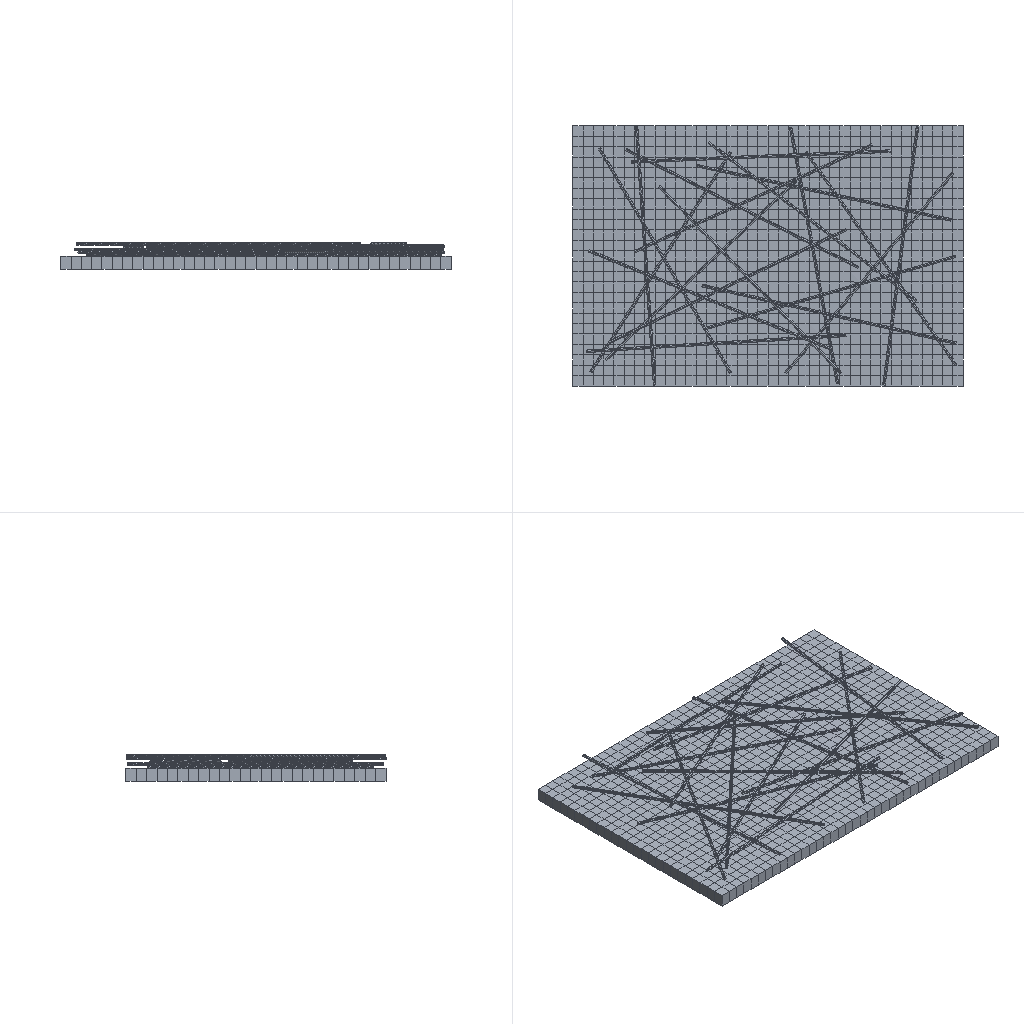Simulation study | abaqus
Set-up summary:
category,name,step,type,value,unit,region
solver,abaqus
solver,version,,,Abaqus/Explicit 2020
units,not stated in the deck,,not stated
analysis,deck,,transient,transient
load_step,Step-1,Step-1,transient
load_step,Step-2,Step-2,transient
load_step,requested,,,2
mesh,nodes,,,6474
mesh,elements,,,2850
element_type,C3D8R,,solid,2850
load,load commands in deck,,count,3
bc,support commands in deck,,count,18
material,JITI,,in results
material,MATERIAL-1,,in results
check,setup vs results,,match,"per instance, exact: element labels, types and connectivity; labels of the nodes the elements use; coordinates of those nodes at SINGLE_PRECISION in 16 of 20 instance(s)"
Abaqus input file, long lists of numbers shortened:
*Heading
** Job name: Job-2 Model name: Model-1-Copy
** Generated by: Abaqus/CAE 2020
*Preprint, echo=NO, model=NO, history=NO, contact=NO
**
** PARTS
**
*Part, name=P1111-1
*End Part
**
*Part, name=P1111-2
*End Part
**
*Part, name=P1111-3
*End Part
**
*Part, name=P1111-4
*End Part
**
*Part, name=P1111-5
*End Part
**
*Part, name=P1111-6
*End Part
**
*Part, name=P1111-7
*End Part
**
*Part, name=P1111-8
*End Part
**
*Part, name=P1111-9
*End Part
**
*Part, name=P1111-10
*End Part
**
*Part, name=P1111-11
*End Part
**
*Part, name=P1111-12
*End Part
**
*Part, name=P1111-13
*End Part
**
*Part, name=P1111-14
*End Part
**
*Part, name=P1111-15
*End Part
**
*Part, name=P1111-16
*End Part
**
*Part, name=P1111-17
*End Part
**
*Part, name=P1111-18
*End Part
**
*Part, name=P1111-19
*End Part
**
*Part, name=P1111-20
*End Part
**
**
** ASSEMBLY
**
*Assembly, name=Assembly
**
*Instance, name=P1111-1-1, part=P1111-1
*Node
      1,  -42.19,   54.229,           0.
      2,  -42.19,   50.229,           0.
** (2026 more lines like these left out)
*Element, type=C3D8R
  1,   53,   54,   80,   79,    1,    2,   28,   27
  2,   54,   55,   81,   80,    2,    3,   29,   28
** (948 more lines like these left out)
*Nset, nset=Set-1, generate
    1,  2028,     1
*Elset, elset=Set-1, generate
   1,  950,    1
** Section: jiti
*Solid Section, elset=Set-1, material=jiti
,
*End Instance
**
*Instance, name=P1111-2-1, part=P1111-2
*Node
      1,  -31.669,   45.76,   5.139
      2,  -31.974,   45.582,   4.992
** (232 more lines like these left out)
*Element, type=C3D8R
  1,   1,   9,   3,   2,  10,  18,  12,  11
  2,   7,   6,   5,   9,  16,  15,  14,  18
** (98 more lines like these left out)
*Nset, nset=Set-1, generate
   1,  234,    1
*Elset, elset=Set-1, generate
   1,  100,    1
** Section: yuanzhu
*Solid Section, elset=Set-1, material=Material-1
,
*End Instance
**
*Instance, name=P1111-3-1, part=P1111-3
*Node
      1,   104.08,   35.777,   5.139
      2,    103.809,   36.004,   4.992
** (232 more lines like these left out)
*Element, type=C3D8R
  1,   2,   1,   8,   9,  11,  10,  17,  18
  2,   2,   9,   4,   3,  11,  18,  13,  12
** (98 more lines like these left out)
*Nset, nset=Set-1, generate
   1,  234,    1
*Elset, elset=Set-1, generate
   1,  100,    1
** Section: yuanzhu
*Solid Section, elset=Set-1, material=Material-1
,
*End Instance
**
*Instance, name=P1111-4-1, part=P1111-4
*Node
      1,  -21.552,   45.409,   5.139
      2,  -21.712,   45.094,   4.992
** (232 more lines like these left out)
*Element, type=C3D8R
  1,   6,   9,   8,   7,  15,  18,  17,  16
  2,   4,   3,   2,   9,  13,  12,  11,  18
** (98 more lines like these left out)
*Nset, nset=Set-1, generate
   1,  234,    1
*Elset, elset=Set-1, generate
   1,  100,    1
** Section: yuanzhu
*Solid Section, elset=Set-1, material=Material-1
,
*End Instance
**
*Instance, name=P1111-5-1, part=P1111-5
*Node
      1,   -35.497,  -40.087,   6.265
      2,  -35.199,  -40.277,   6.118
** (232 more lines like these left out)
*Element, type=C3D8R
  1,   4,   9,   6,   5,  13,  18,  15,  14
  2,   8,   7,   6,   9,  17,  16,  15,  18
** (98 more lines like these left out)
*Nset, nset=Set-1, generate
   1,  234,    1
*Elset, elset=Set-1, generate
   1,  100,    1
** Section: yuanzhu
*Solid Section, elset=Set-1, material=Material-1
,
*End Instance
**
*Instance, name=P1111-6-1, part=P1111-6
*Node
      1,   104.726,  -37.897,   6.265
      2,   105.015,  -37.693,   6.118
** (232 more lines like these left out)
*Element, type=C3D8R
  1,   6,   9,   8,   7,  15,  18,  17,  16
  2,   6,   5,   4,   9,  15,  14,  13,  18
** (98 more lines like these left out)
*Nset, nset=Set-1, generate
   1,  234,    1
*Elset, elset=Set-1, generate
   1,  100,    1
** Section: yuanzhu
*Solid Section, elset=Set-1, material=Material-1
,
*End Instance
**
*Instance, name=P1111-7-1, part=P1111-7
*Node
      1,   59.185,  -44.893,   6.265
      2,   59.533,  -44.83,   6.118
** (232 more lines like these left out)
*Element, type=C3D8R
  1,   4,   3,   2,   9,  13,  12,  11,  18
  2,   4,   9,   6,   5,  13,  18,  15,  14
** (98 more lines like these left out)
*Nset, nset=Set-1, generate
   1,  234,    1
*Elset, elset=Set-1, generate
   1,  100,    1
** Section: yuanzhu
*Solid Section, elset=Set-1, material=Material-1
,
*End Instance
**
*Instance, name=P1111-8-1, part=P1111-8
*Node
      1,  -29.698,  -35.221,   6.303
      2,   -29.456,  -35.479,    6.156
** (232 more lines like these left out)
*Element, type=C3D8R
  1,   8,   7,   6,   9,  17,  16,  15,  18
  2,   8,   9,   2,   1,  17,  18,  11,  10
** (98 more lines like these left out)
*Nset, nset=Set-1, generate
   1,  234,    1
*Elset, elset=Set-1, generate
   1,  100,    1
** Section: yuanzhu
*Solid Section, elset=Set-1, material=Material-1
,
*End Instance
**
*Instance, name=P1111-9-1, part=P1111-9
*Node
      1,  -37.063,  -32.075,   7.313
      2,  -37.041,  -32.428,   7.166
** (232 more lines like these left out)
*Element, type=C3D8R
  1,   6,   9,   8,   7,  15,  18,  17,  16
  2,   4,   3,   2,   9,  13,  12,  11,  18
** (98 more lines like these left out)
*Nset, nset=Set-1, generate
   1,  234,    1
*Elset, elset=Set-1, generate
   1,  100,    1
** Section: yuanzhu
*Solid Section, elset=Set-1, material=Material-1
,
*End Instance
**
*Instance, name=P1111-10-1, part=P1111-10
*Node
      1,  -27.663,  -28.386,   7.313
      2,  -27.511,  -28.705,   7.166
** (232 more lines like these left out)
*Element, type=C3D8R
  1,   2,   1,   8,   9,  11,  10,  17,  18
  2,   4,   9,   6,   5,  13,  18,  15,  14
** (98 more lines like these left out)
*Nset, nset=Set-1, generate
   1,  234,    1
*Elset, elset=Set-1, generate
   1,  100,    1
** Section: yuanzhu
*Solid Section, elset=Set-1, material=Material-1
,
*End Instance
**
*Instance, name=P1111-11-1, part=P1111-11
*Node
      1,   5.398,   39.306,   7.313
      2,   5.324,   38.96,   7.166
** (232 more lines like these left out)
*Element, type=C3D8R
  1,   6,   9,   8,   7,  15,  18,  17,  16
  2,   8,   9,   2,   1,  17,  18,  11,  10
** (98 more lines like these left out)
*Nset, nset=Set-1, generate
   1,  234,    1
*Elset, elset=Set-1, generate
   1,  100,    1
** Section: yuanzhu
*Solid Section, elset=Set-1, material=Material-1
,
*End Instance
**
*Instance, name=P1111-12-1, part=P1111-12
*Node
      1,   7.535,  -6.803,   8.533
      2,   7.456,  -7.148,    8.386
** (232 more lines like these left out)
*Element, type=C3D8R
  1,   5,   9,   7,   6,  14,  18,  16,  15
  2,   1,   8,   7,   9,  10,  17,  16,  18
** (98 more lines like these left out)
*Nset, nset=Set-1, generate
   1,  234,    1
*Elset, elset=Set-1, generate
   1,  100,    1
** Section: yuanzhu
*Solid Section, elset=Set-1, material=Material-1
,
*End Instance
**
*Instance, name=P1111-13-1, part=P1111-13
*Node
      1,  -8.713,   31.118,   8.404
      2,  -8.966,    30.871,   8.258
** (232 more lines like these left out)
*Element, type=C3D8R
  1,   4,   9,   6,   5,  13,  18,  15,  14
  2,   8,   9,   2,   1,  17,  18,  11,  10
** (98 more lines like these left out)
*Nset, nset=Set-1, generate
   1,  234,    1
*Elset, elset=Set-1, generate
   1,  100,    1
** Section: yuanzhu
*Solid Section, elset=Set-1, material=Material-1
,
*End Instance
**
*Instance, name=P1111-14-1, part=P1111-14
*Node
      1,   90.585,   53.756,   9.437
      2,   90.235,   53.802,   9.29
** (232 more lines like these left out)
*Element, type=C3D8R
  1,   5,   9,   7,   6,  14,  18,  16,  15
  2,   1,   9,   3,   2,  10,  18,  12,  11
** (98 more lines like these left out)
*Nset, nset=Set-1, generate
   1,  234,    1
*Elset, elset=Set-1, generate
   1,  100,    1
** Section: yuanzhu
*Solid Section, elset=Set-1, material=Material-1
,
*End Instance
**
*Instance, name=P1111-15-1, part=P1111-15
*Node
      1,  -17.369,   53.979,   8.404
      2,  -17.722,    53.955,   8.258
** (232 more lines like these left out)
*Element, type=C3D8R
  1,   7,   6,   5,   9,  16,  15,  14,  18
  2,   5,   4,   3,   9,  14,  13,  12,  18
** (98 more lines like these left out)
*Nset, nset=Set-1, generate
   1,  234,    1
*Elset, elset=Set-1, generate
   1,  100,    1
** Section: yuanzhu
*Solid Section, elset=Set-1, material=Material-1
,
*End Instance
**
*Instance, name=P1111-16-1, part=P1111-16
*Node
      1,   10.313,   47.989,   8.404
      2,   10.099,   47.707,   8.258
** (232 more lines like these left out)
*Element, type=C3D8R
  1,   1,   9,   3,   2,  10,  18,  12,  11
  2,   7,   6,   5,   9,  16,  15,  14,  18
** (98 more lines like these left out)
*Nset, nset=Set-1, generate
   1,  234,    1
*Elset, elset=Set-1, generate
   1,  100,    1
** Section: yuanzhu
*Solid Section, elset=Set-1, material=Material-1
,
*End Instance
**
*Instance, name=P1111-17-1, part=P1111-17
*Node
      1,  -35.913,   6.512,   9.437
      2,   -36.045,   6.185,   9.29
** (232 more lines like these left out)
*Element, type=C3D8R
  1,   5,   9,   7,   6,  14,  18,  16,  15
  2,   5,   4,   3,   9,  14,  13,  12,  18
** (98 more lines like these left out)
*Nset, nset=Set-1, generate
   1,  234,    1
*Elset, elset=Set-1, generate
   1,  100,    1
** Section: yuanzhu
*Solid Section, elset=Set-1, material=Material-1
,
*End Instance
**
*Instance, name=P1111-18-1, part=P1111-18
*Node
      1,  -18.626,   6.193,   9.437
      2,  -18.481,   5.871,   9.29
** (232 more lines like these left out)
*Element, type=C3D8R
  1,   7,   6,   5,   9,  16,  15,  14,  18
  2,   1,   8,   7,   9,  10,  17,  16,  18
** (98 more lines like these left out)
*Nset, nset=Set-1, generate
   1,  234,    1
*Elset, elset=Set-1, generate
   1,  100,    1
** Section: yuanzhu
*Solid Section, elset=Set-1, material=Material-1
,
*End Instance
**
*Instance, name=P1111-19-1, part=P1111-19
*Node
      1,  -19.828,   40.731,   7.313
      2,  -19.814,   40.378,   7.166
** (232 more lines like these left out)
*Element, type=C3D8R
  1,   1,   9,   3,   2,  10,  18,  12,  11
  2,   7,   6,   5,   9,  16,  15,  14,  18
** (98 more lines like these left out)
*Nset, nset=Set-1, generate
   1,  234,    1
*Elset, elset=Set-1, generate
   1,  100,    1
** Section: yuanzhu
*Solid Section, elset=Set-1, material=Material-1
,
*End Instance
**
*Instance, name=P1111-20-1, part=P1111-20
*Node
      1,   8.641,  -23.322,   7.313
      2,   8.739,   -23.661,   7.166
** (232 more lines like these left out)
*Element, type=C3D8R
  1,   2,   1,   8,   9,  11,  10,  17,  18
  2,   4,   9,   6,   5,  13,  18,  15,  14
** (98 more lines like these left out)
*Nset, nset=Set-1, generate
   1,  234,    1
*Elset, elset=Set-1, generate
   1,  100,    1
** Section: yuanzhu
*Solid Section, elset=Set-1, material=Material-1
,
*End Instance
**
*Nset, nset=Set-1, instance=P1111-2-1, generate
   1,  234,    1
*Nset, nset=Set-1, instance=P1111-3-1, generate
   1,  234,    1
*Nset, nset=Set-1, instance=P1111-4-1, generate
   1,  234,    1
*Nset, nset=Set-1, instance=P1111-8-1, generate
   1,  234,    1
*Nset, nset=Set-1, instance=P1111-16-1, generate
   1,  234,    1
*Nset, nset=Set-1, instance=P1111-12-1, generate
   1,  234,    1
*Nset, nset=Set-1, instance=P1111-20-1, generate
   1,  234,    1
*Nset, nset=Set-1, instance=P1111-6-1, generate
   1,  234,    1
*Nset, nset=Set-1, instance=P1111-10-1, generate
   1,  234,    1
*Nset, nset=Set-1, instance=P1111-18-1, generate
   1,  234,    1
*Nset, nset=Set-1, instance=P1111-14-1, generate
   1,  234,    1
*Nset, nset=Set-1, instance=P1111-5-1, generate
   1,  234,    1
*Nset, nset=Set-1, instance=P1111-9-1, generate
   1,  234,    1
*Nset, nset=Set-1, instance=P1111-17-1, generate
   1,  234,    1
*Nset, nset=Set-1, instance=P1111-13-1, generate
   1,  234,    1
*Nset, nset=Set-1, instance=P1111-7-1, generate
   1,  234,    1
*Nset, nset=Set-1, instance=P1111-11-1, generate
   1,  234,    1
*Nset, nset=Set-1, instance=P1111-19-1, generate
   1,  234,    1
*Nset, nset=Set-1, instance=P1111-15-1, generate
   1,  234,    1
*Elset, elset=Set-1, instance=P1111-2-1, generate
   1,  100,    1
*Elset, elset=Set-1, instance=P1111-3-1, generate
   1,  100,    1
*Elset, elset=Set-1, instance=P1111-4-1, generate
   1,  100,    1
*Elset, elset=Set-1, instance=P1111-8-1, generate
   1,  100,    1
*Elset, elset=Set-1, instance=P1111-16-1, generate
   1,  100,    1
*Elset, elset=Set-1, instance=P1111-12-1, generate
   1,  100,    1
*Elset, elset=Set-1, instance=P1111-20-1, generate
   1,  100,    1
*Elset, elset=Set-1, instance=P1111-6-1, generate
   1,  100,    1
*Elset, elset=Set-1, instance=P1111-10-1, generate
   1,  100,    1
*Elset, elset=Set-1, instance=P1111-18-1, generate
   1,  100,    1
*Elset, elset=Set-1, instance=P1111-14-1, generate
   1,  100,    1
*Elset, elset=Set-1, instance=P1111-5-1, generate
   1,  100,    1
*Elset, elset=Set-1, instance=P1111-9-1, generate
   1,  100,    1
*Elset, elset=Set-1, instance=P1111-17-1, generate
   1,  100,    1
*Elset, elset=Set-1, instance=P1111-13-1, generate
   1,  100,    1
*Elset, elset=Set-1, instance=P1111-7-1, generate
   1,  100,    1
*Elset, elset=Set-1, instance=P1111-11-1, generate
   1,  100,    1
*Elset, elset=Set-1, instance=P1111-19-1, generate
   1,  100,    1
*Elset, elset=Set-1, instance=P1111-15-1, generate
   1,  100,    1
*Nset, nset=Set-2, instance=P1111-1-1, generate
  1,  52,   1
*Elset, elset=Set-2, instance=P1111-1-1, generate
  1,  25,   1
*Nset, nset=Set-3, instance=P1111-1-1, generate
 1977,  2028,     1
*Elset, elset=Set-3, instance=P1111-1-1, generate
 926,  950,    1
*Nset, nset=Set-4, instance=P1111-1-1
    1,    2,    3,    4,    5,    6,    7,    8,    9,   10,   11,   12,   13,   14,   15,   16
   17,   18,   19,   20,   21,   22,   23,   24,   25,   26,   53,   54,   55,   56,   57,   58
** (62 more lines like these left out)
*Elset, elset=Set-4, instance=P1111-1-1, generate
   1,  950,    1
*Elset, elset=_m_Surf-1_S5, internal, instance=P1111-2-1, generate
  1,  97,   4
*Elset, elset=_m_Surf-1_S5, internal, instance=P1111-3-1
  2,  3,  6,  7, 10, 11, 14, 15, 18, 19, 22, 23, 26, 27, 30, 31
 34, 35, 38, 39, 42, 43, 46, 47, 50, 51, 54, 55, 58, 59, 62, 63
** (2 more lines like these left out)
*Elset, elset=_m_Surf-1_S5, internal, instance=P1111-4-1
   1,   3,   4,   5,   7,   8,   9,  11,  12,  13,  15,  16,  17,  19,  20,  21
  23,  24,  25,  27,  28,  29,  31,  32,  33,  35,  36,  37,  39,  40,  41,  43
** (3 more lines like these left out)
*Elset, elset=_m_Surf-1_S5, internal, instance=P1111-8-1
   2,   3,   4,   6,   7,   8,  10,  11,  12,  14,  15,  16,  18,  19,  20,  22
  23,  24,  26,  27,  28,  30,  31,  32,  34,  35,  36,  38,  39,  40,  42,  43
** (3 more lines like these left out)
*Elset, elset=_m_Surf-1_S5, internal, instance=P1111-16-1, generate
  1,  99,   2
*Elset, elset=_m_Surf-1_S5, internal, instance=P1111-12-1
   1,   4,   5,   8,   9,  12,  13,  16,  17,  20,  21,  24,  25,  28,  29,  32
  33,  36,  37,  40,  41,  44,  45,  48,  49,  52,  53,  56,  57,  60,  61,  64
** (2 more lines like these left out)
*Elset, elset=_m_Surf-1_S5, internal, instance=P1111-20-1
  2,  3,  6,  7, 10, 11, 14, 15, 18, 19, 22, 23, 26, 27, 30, 31
 34, 35, 38, 39, 42, 43, 46, 47, 50, 51, 54, 55, 58, 59, 62, 63
** (2 more lines like these left out)
*Elset, elset=_m_Surf-1_S5, internal, instance=P1111-6-1
   1,   3,   4,   5,   7,   8,   9,  11,  12,  13,  15,  16,  17,  19,  20,  21
  23,  24,  25,  27,  28,  29,  31,  32,  33,  35,  36,  37,  39,  40,  41,  43
** (3 more lines like these left out)
*Elset, elset=_m_Surf-1_S5, internal, instance=P1111-10-1
  2,  3,  6,  7, 10, 11, 14, 15, 18, 19, 22, 23, 26, 27, 30, 31
 34, 35, 38, 39, 42, 43, 46, 47, 50, 51, 54, 55, 58, 59, 62, 63
** (2 more lines like these left out)
*Elset, elset=_m_Surf-1_S5, internal, instance=P1111-18-1, generate
  3,  99,   4
*Elset, elset=_m_Surf-1_S5, internal, instance=P1111-14-1
  1,  2,  3,  5,  6,  7,  9, 10, 11, 13, 14, 15, 17, 18, 19, 21
 22, 23, 25, 26, 27, 29, 30, 31, 33, 34, 35, 37, 38, 39, 41, 42
** (3 more lines like these left out)
*Elset, elset=_m_Surf-1_S5, internal, instance=P1111-5-1, generate
  1,  97,   4
*Elset, elset=_m_Surf-1_S5, internal, instance=P1111-9-1
   1,   3,   4,   5,   7,   8,   9,  11,  12,  13,  15,  16,  17,  19,  20,  21
  23,  24,  25,  27,  28,  29,  31,  32,  33,  35,  36,  37,  39,  40,  41,  43
** (3 more lines like these left out)
*Elset, elset=_m_Surf-1_S5, internal, instance=P1111-17-1
   1,   4,   5,   8,   9,  12,  13,  16,  17,  20,  21,  24,  25,  28,  29,  32
  33,  36,  37,  40,  41,  44,  45,  48,  49,  52,  53,  56,  57,  60,  61,  64
** (2 more lines like these left out)
*Elset, elset=_m_Surf-1_S5, internal, instance=P1111-13-1
  1,  2,  3,  5,  6,  7,  9, 10, 11, 13, 14, 15, 17, 18, 19, 21
 22, 23, 25, 26, 27, 29, 30, 31, 33, 34, 35, 37, 38, 39, 41, 42
** (3 more lines like these left out)
*Elset, elset=_m_Surf-1_S5, internal, instance=P1111-7-1, generate
  2,  98,   4
*Elset, elset=_m_Surf-1_S5, internal, instance=P1111-11-1, generate
   1,  100,    1
*Elset, elset=_m_Surf-1_S5, internal, instance=P1111-19-1, generate
  1,  99,   2
*Elset, elset=_m_Surf-1_S5, internal, instance=P1111-15-1, generate
   4,  100,    4
*Elset, elset=_m_Surf-1_S6, internal, instance=P1111-2-1, generate
  1,  97,   4
*Elset, elset=_m_Surf-1_S6, internal, instance=P1111-3-1
  2,  3,  6,  7, 10, 11, 14, 15, 18, 19, 22, 23, 26, 27, 30, 31
 34, 35, 38, 39, 42, 43, 46, 47, 50, 51, 54, 55, 58, 59, 62, 63
** (2 more lines like these left out)
*Elset, elset=_m_Surf-1_S6, internal, instance=P1111-4-1
   1,   3,   4,   5,   7,   8,   9,  11,  12,  13,  15,  16,  17,  19,  20,  21
  23,  24,  25,  27,  28,  29,  31,  32,  33,  35,  36,  37,  39,  40,  41,  43
** (3 more lines like these left out)
*Elset, elset=_m_Surf-1_S6, internal, instance=P1111-8-1
   2,   3,   4,   6,   7,   8,  10,  11,  12,  14,  15,  16,  18,  19,  20,  22
  23,  24,  26,  27,  28,  30,  31,  32,  34,  35,  36,  38,  39,  40,  42,  43
** (3 more lines like these left out)
*Elset, elset=_m_Surf-1_S6, internal, instance=P1111-16-1, generate
  1,  99,   2
*Elset, elset=_m_Surf-1_S6, internal, instance=P1111-12-1
   1,   4,   5,   8,   9,  12,  13,  16,  17,  20,  21,  24,  25,  28,  29,  32
  33,  36,  37,  40,  41,  44,  45,  48,  49,  52,  53,  56,  57,  60,  61,  64
** (2 more lines like these left out)
*Elset, elset=_m_Surf-1_S6, internal, instance=P1111-20-1
  2,  3,  6,  7, 10, 11, 14, 15, 18, 19, 22, 23, 26, 27, 30, 31
 34, 35, 38, 39, 42, 43, 46, 47, 50, 51, 54, 55, 58, 59, 62, 63
** (2 more lines like these left out)
*Elset, elset=_m_Surf-1_S6, internal, instance=P1111-6-1
   1,   3,   4,   5,   7,   8,   9,  11,  12,  13,  15,  16,  17,  19,  20,  21
  23,  24,  25,  27,  28,  29,  31,  32,  33,  35,  36,  37,  39,  40,  41,  43
** (3 more lines like these left out)
*Elset, elset=_m_Surf-1_S6, internal, instance=P1111-10-1
  2,  3,  6,  7, 10, 11, 14, 15, 18, 19, 22, 23, 26, 27, 30, 31
 34, 35, 38, 39, 42, 43, 46, 47, 50, 51, 54, 55, 58, 59, 62, 63
** (2 more lines like these left out)
*Elset, elset=_m_Surf-1_S6, internal, instance=P1111-18-1, generate
  3,  99,   4
*Elset, elset=_m_Surf-1_S6, internal, instance=P1111-14-1
  1,  2,  3,  5,  6,  7,  9, 10, 11, 13, 14, 15, 17, 18, 19, 21
 22, 23, 25, 26, 27, 29, 30, 31, 33, 34, 35, 37, 38, 39, 41, 42
** (3 more lines like these left out)
*Elset, elset=_m_Surf-1_S6, internal, instance=P1111-5-1, generate
  1,  97,   4
*Elset, elset=_m_Surf-1_S6, internal, instance=P1111-9-1
   1,   3,   4,   5,   7,   8,   9,  11,  12,  13,  15,  16,  17,  19,  20,  21
  23,  24,  25,  27,  28,  29,  31,  32,  33,  35,  36,  37,  39,  40,  41,  43
** (3 more lines like these left out)
*Elset, elset=_m_Surf-1_S6, internal, instance=P1111-17-1
   1,   4,   5,   8,   9,  12,  13,  16,  17,  20,  21,  24,  25,  28,  29,  32
  33,  36,  37,  40,  41,  44,  45,  48,  49,  52,  53,  56,  57,  60,  61,  64
** (2 more lines like these left out)
*Elset, elset=_m_Surf-1_S6, internal, instance=P1111-13-1
  1,  2,  3,  5,  6,  7,  9, 10, 11, 13, 14, 15, 17, 18, 19, 21
 22, 23, 25, 26, 27, 29, 30, 31, 33, 34, 35, 37, 38, 39, 41, 42
** (3 more lines like these left out)
*Elset, elset=_m_Surf-1_S6, internal, instance=P1111-7-1, generate
  2,  98,   4
*Elset, elset=_m_Surf-1_S6, internal, instance=P1111-11-1, generate
   1,  100,    1
*Elset, elset=_m_Surf-1_S6, internal, instance=P1111-19-1, generate
  1,  99,   2
*Elset, elset=_m_Surf-1_S6, internal, instance=P1111-15-1, generate
   4,  100,    4
*Elset, elset=_m_Surf-1_S3, internal, instance=P1111-2-1
   2,   3,   4,   6,   7,   8,  10,  11,  12,  14,  15,  16,  18,  19,  20,  22
  23,  24,  26,  27,  28,  30,  31,  32,  34,  35,  36,  38,  39,  40,  42,  43
** (3 more lines like these left out)
*Elset, elset=_m_Surf-1_S3, internal, instance=P1111-3-1
   1,   4,   5,   8,   9,  12,  13,  16,  17,  20,  21,  24,  25,  28,  29,  32
  33,  36,  37,  40,  41,  44,  45,  48,  49,  52,  53,  56,  57,  60,  61,  64
** (2 more lines like these left out)
*Elset, elset=_m_Surf-1_S3, internal, instance=P1111-4-1, generate
  2,  98,   4
*Elset, elset=_m_Surf-1_S3, internal, instance=P1111-8-1, generate
  1,  97,   4
*Elset, elset=_m_Surf-1_S3, internal, instance=P1111-16-1, generate
   2,  100,    2
*Elset, elset=_m_Surf-1_S3, internal, instance=P1111-12-1
  2,  3,  6,  7, 10, 11, 14, 15, 18, 19, 22, 23, 26, 27, 30, 31
 34, 35, 38, 39, 42, 43, 46, 47, 50, 51, 54, 55, 58, 59, 62, 63
** (2 more lines like these left out)
*Elset, elset=_m_Surf-1_S3, internal, instance=P1111-20-1
   1,   4,   5,   8,   9,  12,  13,  16,  17,  20,  21,  24,  25,  28,  29,  32
  33,  36,  37,  40,  41,  44,  45,  48,  49,  52,  53,  56,  57,  60,  61,  64
** (2 more lines like these left out)
*Elset, elset=_m_Surf-1_S3, internal, instance=P1111-6-1, generate
  2,  98,   4
*Elset, elset=_m_Surf-1_S3, internal, instance=P1111-10-1
   1,   4,   5,   8,   9,  12,  13,  16,  17,  20,  21,  24,  25,  28,  29,  32
  33,  36,  37,  40,  41,  44,  45,  48,  49,  52,  53,  56,  57,  60,  61,  64
** (2 more lines like these left out)
*Elset, elset=_m_Surf-1_S3, internal, instance=P1111-18-1
   1,   2,   4,   5,   6,   8,   9,  10,  12,  13,  14,  16,  17,  18,  20,  21
  22,  24,  25,  26,  28,  29,  30,  32,  33,  34,  36,  37,  38,  40,  41,  42
** (3 more lines like these left out)
*Elset, elset=_m_Surf-1_S3, internal, instance=P1111-14-1, generate
   4,  100,    4
*Elset, elset=_m_Surf-1_S3, internal, instance=P1111-5-1
   2,   3,   4,   6,   7,   8,  10,  11,  12,  14,  15,  16,  18,  19,  20,  22
  23,  24,  26,  27,  28,  30,  31,  32,  34,  35,  36,  38,  39,  40,  42,  43
** (3 more lines like these left out)
*Elset, elset=_m_Surf-1_S3, internal, instance=P1111-9-1, generate
  2,  98,   4
*Elset, elset=_m_Surf-1_S3, internal, instance=P1111-17-1
  2,  3,  6,  7, 10, 11, 14, 15, 18, 19, 22, 23, 26, 27, 30, 31
 34, 35, 38, 39, 42, 43, 46, 47, 50, 51, 54, 55, 58, 59, 62, 63
** (2 more lines like these left out)
*Elset, elset=_m_Surf-1_S3, internal, instance=P1111-13-1, generate
   4,  100,    4
*Elset, elset=_m_Surf-1_S3, internal, instance=P1111-7-1
   1,   3,   4,   5,   7,   8,   9,  11,  12,  13,  15,  16,  17,  19,  20,  21
  23,  24,  25,  27,  28,  29,  31,  32,  33,  35,  36,  37,  39,  40,  41,  43
** (3 more lines like these left out)
*Elset, elset=_m_Surf-1_S3, internal, instance=P1111-19-1, generate
   2,  100,    2
*Elset, elset=_m_Surf-1_S3, internal, instance=P1111-15-1
  1,  2,  3,  5,  6,  7,  9, 10, 11, 13, 14, 15, 17, 18, 19, 21
 22, 23, 25, 26, 27, 29, 30, 31, 33, 34, 35, 37, 38, 39, 41, 42
** (3 more lines like these left out)
*Elset, elset=_m_Surf-1_S4, internal, instance=P1111-2-1
   2,   3,   4,   6,   7,   8,  10,  11,  12,  14,  15,  16,  18,  19,  20,  22
  23,  24,  26,  27,  28,  30,  31,  32,  34,  35,  36,  38,  39,  40,  42,  43
** (3 more lines like these left out)
*Elset, elset=_m_Surf-1_S4, internal, instance=P1111-3-1
   1,   4,   5,   8,   9,  12,  13,  16,  17,  20,  21,  24,  25,  28,  29,  32
  33,  36,  37,  40,  41,  44,  45,  48,  49,  52,  53,  56,  57,  60,  61,  64
** (2 more lines like these left out)
*Elset, elset=_m_Surf-1_S4, internal, instance=P1111-4-1, generate
  2,  98,   4
*Elset, elset=_m_Surf-1_S4, internal, instance=P1111-8-1, generate
  1,  97,   4
*Elset, elset=_m_Surf-1_S4, internal, instance=P1111-16-1, generate
   2,  100,    2
*Elset, elset=_m_Surf-1_S4, internal, instance=P1111-12-1
  2,  3,  6,  7, 10, 11, 14, 15, 18, 19, 22, 23, 26, 27, 30, 31
 34, 35, 38, 39, 42, 43, 46, 47, 50, 51, 54, 55, 58, 59, 62, 63
** (2 more lines like these left out)
*Elset, elset=_m_Surf-1_S4, internal, instance=P1111-20-1
   1,   4,   5,   8,   9,  12,  13,  16,  17,  20,  21,  24,  25,  28,  29,  32
  33,  36,  37,  40,  41,  44,  45,  48,  49,  52,  53,  56,  57,  60,  61,  64
** (2 more lines like these left out)
*Elset, elset=_m_Surf-1_S4, internal, instance=P1111-6-1, generate
  2,  98,   4
*Elset, elset=_m_Surf-1_S4, internal, instance=P1111-10-1
   1,   4,   5,   8,   9,  12,  13,  16,  17,  20,  21,  24,  25,  28,  29,  32
  33,  36,  37,  40,  41,  44,  45,  48,  49,  52,  53,  56,  57,  60,  61,  64
** (2 more lines like these left out)
*Elset, elset=_m_Surf-1_S4, internal, instance=P1111-18-1
   1,   2,   4,   5,   6,   8,   9,  10,  12,  13,  14,  16,  17,  18,  20,  21
  22,  24,  25,  26,  28,  29,  30,  32,  33,  34,  36,  37,  38,  40,  41,  42
** (3 more lines like these left out)
*Elset, elset=_m_Surf-1_S4, internal, instance=P1111-14-1, generate
   4,  100,    4
*Elset, elset=_m_Surf-1_S4, internal, instance=P1111-5-1
   2,   3,   4,   6,   7,   8,  10,  11,  12,  14,  15,  16,  18,  19,  20,  22
  23,  24,  26,  27,  28,  30,  31,  32,  34,  35,  36,  38,  39,  40,  42,  43
** (3 more lines like these left out)
*Elset, elset=_m_Surf-1_S4, internal, instance=P1111-9-1, generate
  2,  98,   4
*Elset, elset=_m_Surf-1_S4, internal, instance=P1111-17-1
  2,  3,  6,  7, 10, 11, 14, 15, 18, 19, 22, 23, 26, 27, 30, 31
 34, 35, 38, 39, 42, 43, 46, 47, 50, 51, 54, 55, 58, 59, 62, 63
** (2 more lines like these left out)
*Elset, elset=_m_Surf-1_S4, internal, instance=P1111-13-1, generate
   4,  100,    4
*Elset, elset=_m_Surf-1_S4, internal, instance=P1111-7-1
   1,   3,   4,   5,   7,   8,   9,  11,  12,  13,  15,  16,  17,  19,  20,  21
  23,  24,  25,  27,  28,  29,  31,  32,  33,  35,  36,  37,  39,  40,  41,  43
** (3 more lines like these left out)
*Elset, elset=_m_Surf-1_S4, internal, instance=P1111-19-1, generate
   2,  100,    2
*Elset, elset=_m_Surf-1_S4, internal, instance=P1111-15-1
  1,  2,  3,  5,  6,  7,  9, 10, 11, 13, 14, 15, 17, 18, 19, 21
 22, 23, 25, 26, 27, 29, 30, 31, 33, 34, 35, 37, 38, 39, 41, 42
** (3 more lines like these left out)
*Elset, elset=_m_Surf-1_S2, internal, instance=P1111-2-1, generate
  97,  100,    1
*Elset, elset=_m_Surf-1_S2, internal, instance=P1111-3-1, generate
  97,  100,    1
*Elset, elset=_m_Surf-1_S2, internal, instance=P1111-4-1, generate
  97,  100,    1
*Elset, elset=_m_Surf-1_S2, internal, instance=P1111-8-1, generate
  97,  100,    1
*Elset, elset=_m_Surf-1_S2, internal, instance=P1111-16-1, generate
  97,  100,    1
*Elset, elset=_m_Surf-1_S2, internal, instance=P1111-12-1, generate
  97,  100,    1
*Elset, elset=_m_Surf-1_S2, internal, instance=P1111-20-1, generate
  97,  100,    1
*Elset, elset=_m_Surf-1_S2, internal, instance=P1111-6-1, generate
  97,  100,    1
*Elset, elset=_m_Surf-1_S2, internal, instance=P1111-10-1, generate
  97,  100,    1
*Elset, elset=_m_Surf-1_S2, internal, instance=P1111-18-1, generate
  97,  100,    1
*Elset, elset=_m_Surf-1_S2, internal, instance=P1111-14-1, generate
  97,  100,    1
*Elset, elset=_m_Surf-1_S2, internal, instance=P1111-5-1, generate
  97,  100,    1
*Elset, elset=_m_Surf-1_S2, internal, instance=P1111-9-1, generate
  97,  100,    1
*Elset, elset=_m_Surf-1_S2, internal, instance=P1111-17-1, generate
  97,  100,    1
*Elset, elset=_m_Surf-1_S2, internal, instance=P1111-13-1, generate
  97,  100,    1
*Elset, elset=_m_Surf-1_S2, internal, instance=P1111-7-1, generate
  97,  100,    1
*Elset, elset=_m_Surf-1_S2, internal, instance=P1111-11-1, generate
  97,  100,    1
*Elset, elset=_m_Surf-1_S2, internal, instance=P1111-19-1, generate
  97,  100,    1
*Elset, elset=_m_Surf-1_S2, internal, instance=P1111-15-1, generate
  97,  100,    1
*Elset, elset=_m_Surf-1_S1, internal, instance=P1111-2-1, generate
 1,  4,  1
*Elset, elset=_m_Surf-1_S1, internal, instance=P1111-3-1, generate
 1,  4,  1
*Elset, elset=_m_Surf-1_S1, internal, instance=P1111-4-1, generate
 1,  4,  1
*Elset, elset=_m_Surf-1_S1, internal, instance=P1111-8-1, generate
 1,  4,  1
*Elset, elset=_m_Surf-1_S1, internal, instance=P1111-16-1, generate
 1,  4,  1
*Elset, elset=_m_Surf-1_S1, internal, instance=P1111-12-1, generate
 1,  4,  1
*Elset, elset=_m_Surf-1_S1, internal, instance=P1111-20-1, generate
 1,  4,  1
*Elset, elset=_m_Surf-1_S1, internal, instance=P1111-6-1, generate
 1,  4,  1
*Elset, elset=_m_Surf-1_S1, internal, instance=P1111-10-1, generate
 1,  4,  1
*Elset, elset=_m_Surf-1_S1, internal, instance=P1111-18-1, generate
 1,  4,  1
*Elset, elset=_m_Surf-1_S1, internal, instance=P1111-14-1, generate
 1,  4,  1
*Elset, elset=_m_Surf-1_S1, internal, instance=P1111-5-1, generate
 1,  4,  1
*Elset, elset=_m_Surf-1_S1, internal, instance=P1111-9-1, generate
 1,  4,  1
*Elset, elset=_m_Surf-1_S1, internal, instance=P1111-17-1, generate
 1,  4,  1
*Elset, elset=_m_Surf-1_S1, internal, instance=P1111-13-1, generate
 1,  4,  1
*Elset, elset=_m_Surf-1_S1, internal, instance=P1111-7-1, generate
 1,  4,  1
*Elset, elset=_m_Surf-1_S1, internal, instance=P1111-11-1, generate
 1,  4,  1
*Elset, elset=_m_Surf-1_S1, internal, instance=P1111-19-1, generate
 1,  4,  1
*Elset, elset=_m_Surf-1_S1, internal, instance=P1111-15-1, generate
 1,  4,  1
*Surface, type=ELEMENT, name=m_Surf-1
_m_Surf-1_S5, S5
_m_Surf-1_S6, S6
_m_Surf-1_S4, S4
_m_Surf-1_S2, S2
_m_Surf-1_S3, S3
_m_Surf-1_S1, S1
*Elset, elset=_m_Surf-3_S3, internal, instance=P1111-15-1
  1,  2,  3,  5,  6,  7,  9, 10, 11, 13, 14, 15, 17, 18, 19, 21
 22, 23, 25, 26, 27, 29, 30, 31, 33, 34, 35, 37, 38, 39, 41, 42
** (3 more lines like these left out)
*Elset, elset=_m_Surf-3_S4, internal, instance=P1111-15-1
  1,  2,  3,  5,  6,  7,  9, 10, 11, 13, 14, 15, 17, 18, 19, 21
 22, 23, 25, 26, 27, 29, 30, 31, 33, 34, 35, 37, 38, 39, 41, 42
** (3 more lines like these left out)
*Elset, elset=_m_Surf-3_S5, internal, instance=P1111-15-1, generate
   4,  100,    4
*Elset, elset=_m_Surf-3_S6, internal, instance=P1111-15-1, generate
   4,  100,    4
*Surface, type=ELEMENT, name=m_Surf-3
_m_Surf-3_S3, S3
_m_Surf-3_S4, S4
_m_Surf-3_S6, S6
_m_Surf-3_S5, S5
*Elset, elset=_m_Surf-5_S5, internal, instance=P1111-14-1
  1,  2,  3,  5,  6,  7,  9, 10, 11, 13, 14, 15, 17, 18, 19, 21
 22, 23, 25, 26, 27, 29, 30, 31, 33, 34, 35, 37, 38, 39, 41, 42
** (3 more lines like these left out)
*Elset, elset=_m_Surf-5_S6, internal, instance=P1111-14-1
  1,  2,  3,  5,  6,  7,  9, 10, 11, 13, 14, 15, 17, 18, 19, 21
 22, 23, 25, 26, 27, 29, 30, 31, 33, 34, 35, 37, 38, 39, 41, 42
** (3 more lines like these left out)
*Elset, elset=_m_Surf-5_S3, internal, instance=P1111-14-1, generate
   4,  100,    4
*Elset, elset=_m_Surf-5_S4, internal, instance=P1111-14-1, generate
   4,  100,    4
*Surface, type=ELEMENT, name=m_Surf-5
_m_Surf-5_S5, S5
_m_Surf-5_S6, S6
_m_Surf-5_S4, S4
_m_Surf-5_S3, S3
*Elset, elset=_m_Surf-7_S3, internal, instance=P1111-7-1
   1,   3,   4,   5,   7,   8,   9,  11,  12,  13,  15,  16,  17,  19,  20,  21
  23,  24,  25,  27,  28,  29,  31,  32,  33,  35,  36,  37,  39,  40,  41,  43
** (3 more lines like these left out)
*Elset, elset=_m_Surf-7_S4, internal, instance=P1111-7-1
   1,   3,   4,   5,   7,   8,   9,  11,  12,  13,  15,  16,  17,  19,  20,  21
  23,  24,  25,  27,  28,  29,  31,  32,  33,  35,  36,  37,  39,  40,  41,  43
** (3 more lines like these left out)
*Elset, elset=_m_Surf-7_S5, internal, instance=P1111-7-1, generate
  2,  98,   4
*Elset, elset=_m_Surf-7_S6, internal, instance=P1111-7-1, generate
  2,  98,   4
*Surface, type=ELEMENT, name=m_Surf-7
_m_Surf-7_S3, S3
_m_Surf-7_S4, S4
_m_Surf-7_S6, S6
_m_Surf-7_S5, S5
*Elset, elset=_s_Surf-1_S5, internal, instance=P1111-1-1, generate
   1,  950,    1
*Surface, type=ELEMENT, name=s_Surf-1
_s_Surf-1_S5, S5
*Elset, elset=_s_Surf-3_S5, internal, instance=P1111-2-1, generate
  1,  97,   4
*Elset, elset=_s_Surf-3_S5, internal, instance=P1111-4-1
   1,   3,   4,   5,   7,   8,   9,  11,  12,  13,  15,  16,  17,  19,  20,  21
  23,  24,  25,  27,  28,  29,  31,  32,  33,  35,  36,  37,  39,  40,  41,  43
** (3 more lines like these left out)
*Elset, elset=_s_Surf-3_S5, internal, instance=P1111-8-1
   2,   3,   4,   6,   7,   8,  10,  11,  12,  14,  15,  16,  18,  19,  20,  22
  23,  24,  26,  27,  28,  30,  31,  32,  34,  35,  36,  38,  39,  40,  42,  43
** (3 more lines like these left out)
*Elset, elset=_s_Surf-3_S5, internal, instance=P1111-10-1
  2,  3,  6,  7, 10, 11, 14, 15, 18, 19, 22, 23, 26, 27, 30, 31
 34, 35, 38, 39, 42, 43, 46, 47, 50, 51, 54, 55, 58, 59, 62, 63
** (2 more lines like these left out)
*Elset, elset=_s_Surf-3_S5, internal, instance=P1111-18-1, generate
  3,  99,   4
*Elset, elset=_s_Surf-3_S5, internal, instance=P1111-5-1, generate
  1,  97,   4
*Elset, elset=_s_Surf-3_S5, internal, instance=P1111-9-1
   1,   3,   4,   5,   7,   8,   9,  11,  12,  13,  15,  16,  17,  19,  20,  21
  23,  24,  25,  27,  28,  29,  31,  32,  33,  35,  36,  37,  39,  40,  41,  43
** (3 more lines like these left out)
*Elset, elset=_s_Surf-3_S5, internal, instance=P1111-17-1
   1,   4,   5,   8,   9,  12,  13,  16,  17,  20,  21,  24,  25,  28,  29,  32
  33,  36,  37,  40,  41,  44,  45,  48,  49,  52,  53,  56,  57,  60,  61,  64
** (2 more lines like these left out)
*Elset, elset=_s_Surf-3_S5, internal, instance=P1111-19-1, generate
  1,  99,   2
*Elset, elset=_s_Surf-3_S6, internal, instance=P1111-2-1, generate
  1,  97,   4
*Elset, elset=_s_Surf-3_S6, internal, instance=P1111-4-1
   1,   3,   4,   5,   7,   8,   9,  11,  12,  13,  15,  16,  17,  19,  20,  21
  23,  24,  25,  27,  28,  29,  31,  32,  33,  35,  36,  37,  39,  40,  41,  43
** (3 more lines like these left out)
*Elset, elset=_s_Surf-3_S6, internal, instance=P1111-8-1
   2,   3,   4,   6,   7,   8,  10,  11,  12,  14,  15,  16,  18,  19,  20,  22
  23,  24,  26,  27,  28,  30,  31,  32,  34,  35,  36,  38,  39,  40,  42,  43
** (3 more lines like these left out)
*Elset, elset=_s_Surf-3_S6, internal, instance=P1111-10-1
  2,  3,  6,  7, 10, 11, 14, 15, 18, 19, 22, 23, 26, 27, 30, 31
 34, 35, 38, 39, 42, 43, 46, 47, 50, 51, 54, 55, 58, 59, 62, 63
** (2 more lines like these left out)
*Elset, elset=_s_Surf-3_S6, internal, instance=P1111-18-1, generate
  3,  99,   4
*Elset, elset=_s_Surf-3_S6, internal, instance=P1111-5-1, generate
  1,  97,   4
*Elset, elset=_s_Surf-3_S6, internal, instance=P1111-9-1
   1,   3,   4,   5,   7,   8,   9,  11,  12,  13,  15,  16,  17,  19,  20,  21
  23,  24,  25,  27,  28,  29,  31,  32,  33,  35,  36,  37,  39,  40,  41,  43
** (3 more lines like these left out)
*Elset, elset=_s_Surf-3_S6, internal, instance=P1111-17-1
   1,   4,   5,   8,   9,  12,  13,  16,  17,  20,  21,  24,  25,  28,  29,  32
  33,  36,  37,  40,  41,  44,  45,  48,  49,  52,  53,  56,  57,  60,  61,  64
** (2 more lines like these left out)
*Elset, elset=_s_Surf-3_S6, internal, instance=P1111-19-1, generate
  1,  99,   2
*Elset, elset=_s_Surf-3_S3, internal, instance=P1111-2-1
   2,   3,   4,   6,   7,   8,  10,  11,  12,  14,  15,  16,  18,  19,  20,  22
  23,  24,  26,  27,  28,  30,  31,  32,  34,  35,  36,  38,  39,  40,  42,  43
** (3 more lines like these left out)
*Elset, elset=_s_Surf-3_S3, internal, instance=P1111-4-1, generate
  2,  98,   4
*Elset, elset=_s_Surf-3_S3, internal, instance=P1111-8-1, generate
  1,  97,   4
*Elset, elset=_s_Surf-3_S3, internal, instance=P1111-10-1
   1,   4,   5,   8,   9,  12,  13,  16,  17,  20,  21,  24,  25,  28,  29,  32
  33,  36,  37,  40,  41,  44,  45,  48,  49,  52,  53,  56,  57,  60,  61,  64
** (2 more lines like these left out)
*Elset, elset=_s_Surf-3_S3, internal, instance=P1111-18-1
   1,   2,   4,   5,   6,   8,   9,  10,  12,  13,  14,  16,  17,  18,  20,  21
  22,  24,  25,  26,  28,  29,  30,  32,  33,  34,  36,  37,  38,  40,  41,  42
** (3 more lines like these left out)
*Elset, elset=_s_Surf-3_S3, internal, instance=P1111-5-1
   2,   3,   4,   6,   7,   8,  10,  11,  12,  14,  15,  16,  18,  19,  20,  22
  23,  24,  26,  27,  28,  30,  31,  32,  34,  35,  36,  38,  39,  40,  42,  43
** (3 more lines like these left out)
*Elset, elset=_s_Surf-3_S3, internal, instance=P1111-9-1, generate
  2,  98,   4
*Elset, elset=_s_Surf-3_S3, internal, instance=P1111-17-1
  2,  3,  6,  7, 10, 11, 14, 15, 18, 19, 22, 23, 26, 27, 30, 31
 34, 35, 38, 39, 42, 43, 46, 47, 50, 51, 54, 55, 58, 59, 62, 63
** (2 more lines like these left out)
*Elset, elset=_s_Surf-3_S3, internal, instance=P1111-19-1, generate
   2,  100,    2
*Elset, elset=_s_Surf-3_S4, internal, instance=P1111-2-1
   2,   3,   4,   6,   7,   8,  10,  11,  12,  14,  15,  16,  18,  19,  20,  22
  23,  24,  26,  27,  28,  30,  31,  32,  34,  35,  36,  38,  39,  40,  42,  43
** (3 more lines like these left out)
*Elset, elset=_s_Surf-3_S4, internal, instance=P1111-4-1, generate
  2,  98,   4
*Elset, elset=_s_Surf-3_S4, internal, instance=P1111-8-1, generate
  1,  97,   4
*Elset, elset=_s_Surf-3_S4, internal, instance=P1111-10-1
   1,   4,   5,   8,   9,  12,  13,  16,  17,  20,  21,  24,  25,  28,  29,  32
  33,  36,  37,  40,  41,  44,  45,  48,  49,  52,  53,  56,  57,  60,  61,  64
** (2 more lines like these left out)
*Elset, elset=_s_Surf-3_S4, internal, instance=P1111-18-1
   1,   2,   4,   5,   6,   8,   9,  10,  12,  13,  14,  16,  17,  18,  20,  21
  22,  24,  25,  26,  28,  29,  30,  32,  33,  34,  36,  37,  38,  40,  41,  42
** (3 more lines like these left out)
*Elset, elset=_s_Surf-3_S4, internal, instance=P1111-5-1
   2,   3,   4,   6,   7,   8,  10,  11,  12,  14,  15,  16,  18,  19,  20,  22
  23,  24,  26,  27,  28,  30,  31,  32,  34,  35,  36,  38,  39,  40,  42,  43
** (3 more lines like these left out)
*Elset, elset=_s_Surf-3_S4, internal, instance=P1111-9-1, generate
  2,  98,   4
*Elset, elset=_s_Surf-3_S4, internal, instance=P1111-17-1
  2,  3,  6,  7, 10, 11, 14, 15, 18, 19, 22, 23, 26, 27, 30, 31
 34, 35, 38, 39, 42, 43, 46, 47, 50, 51, 54, 55, 58, 59, 62, 63
** (2 more lines like these left out)
*Elset, elset=_s_Surf-3_S4, internal, instance=P1111-19-1, generate
   2,  100,    2
*Surface, type=ELEMENT, name=s_Surf-3
_s_Surf-3_S5, S5
_s_Surf-3_S6, S6
_s_Surf-3_S4, S4
_s_Surf-3_S3, S3
*Elset, elset=_s_Surf-5_S3, internal, instance=P1111-3-1
   1,   4,   5,   8,   9,  12,  13,  16,  17,  20,  21,  24,  25,  28,  29,  32
  33,  36,  37,  40,  41,  44,  45,  48,  49,  52,  53,  56,  57,  60,  61,  64
** (2 more lines like these left out)
*Elset, elset=_s_Surf-5_S3, internal, instance=P1111-6-1, generate
  2,  98,   4
*Elset, elset=_s_Surf-5_S3, internal, instance=P1111-12-1
  2,  3,  6,  7, 10, 11, 14, 15, 18, 19, 22, 23, 26, 27, 30, 31
 34, 35, 38, 39, 42, 43, 46, 47, 50, 51, 54, 55, 58, 59, 62, 63
** (2 more lines like these left out)
*Elset, elset=_s_Surf-5_S3, internal, instance=P1111-16-1, generate
   2,  100,    2
*Elset, elset=_s_Surf-5_S3, internal, instance=P1111-20-1
   1,   4,   5,   8,   9,  12,  13,  16,  17,  20,  21,  24,  25,  28,  29,  32
  33,  36,  37,  40,  41,  44,  45,  48,  49,  52,  53,  56,  57,  60,  61,  64
** (2 more lines like these left out)
*Elset, elset=_s_Surf-5_S4, internal, instance=P1111-3-1
   1,   4,   5,   8,   9,  12,  13,  16,  17,  20,  21,  24,  25,  28,  29,  32
  33,  36,  37,  40,  41,  44,  45,  48,  49,  52,  53,  56,  57,  60,  61,  64
** (2 more lines like these left out)
*Elset, elset=_s_Surf-5_S4, internal, instance=P1111-6-1, generate
  2,  98,   4
*Elset, elset=_s_Surf-5_S4, internal, instance=P1111-12-1
  2,  3,  6,  7, 10, 11, 14, 15, 18, 19, 22, 23, 26, 27, 30, 31
 34, 35, 38, 39, 42, 43, 46, 47, 50, 51, 54, 55, 58, 59, 62, 63
** (2 more lines like these left out)
*Elset, elset=_s_Surf-5_S4, internal, instance=P1111-16-1, generate
   2,  100,    2
*Elset, elset=_s_Surf-5_S4, internal, instance=P1111-20-1
   1,   4,   5,   8,   9,  12,  13,  16,  17,  20,  21,  24,  25,  28,  29,  32
  33,  36,  37,  40,  41,  44,  45,  48,  49,  52,  53,  56,  57,  60,  61,  64
** (2 more lines like these left out)
*Elset, elset=_s_Surf-5_S5, internal, instance=P1111-3-1
  2,  3,  6,  7, 10, 11, 14, 15, 18, 19, 22, 23, 26, 27, 30, 31
 34, 35, 38, 39, 42, 43, 46, 47, 50, 51, 54, 55, 58, 59, 62, 63
** (2 more lines like these left out)
*Elset, elset=_s_Surf-5_S5, internal, instance=P1111-6-1
   1,   3,   4,   5,   7,   8,   9,  11,  12,  13,  15,  16,  17,  19,  20,  21
  23,  24,  25,  27,  28,  29,  31,  32,  33,  35,  36,  37,  39,  40,  41,  43
** (3 more lines like these left out)
*Elset, elset=_s_Surf-5_S5, internal, instance=P1111-12-1
   1,   4,   5,   8,   9,  12,  13,  16,  17,  20,  21,  24,  25,  28,  29,  32
  33,  36,  37,  40,  41,  44,  45,  48,  49,  52,  53,  56,  57,  60,  61,  64
** (2 more lines like these left out)
*Elset, elset=_s_Surf-5_S5, internal, instance=P1111-16-1, generate
  1,  99,   2
*Elset, elset=_s_Surf-5_S5, internal, instance=P1111-20-1
  2,  3,  6,  7, 10, 11, 14, 15, 18, 19, 22, 23, 26, 27, 30, 31
 34, 35, 38, 39, 42, 43, 46, 47, 50, 51, 54, 55, 58, 59, 62, 63
** (2 more lines like these left out)
*Elset, elset=_s_Surf-5_S5, internal, instance=P1111-11-1, generate
   1,  100,    1
*Elset, elset=_s_Surf-5_S6, internal, instance=P1111-3-1
  2,  3,  6,  7, 10, 11, 14, 15, 18, 19, 22, 23, 26, 27, 30, 31
 34, 35, 38, 39, 42, 43, 46, 47, 50, 51, 54, 55, 58, 59, 62, 63
** (2 more lines like these left out)
*Elset, elset=_s_Surf-5_S6, internal, instance=P1111-6-1
   1,   3,   4,   5,   7,   8,   9,  11,  12,  13,  15,  16,  17,  19,  20,  21
  23,  24,  25,  27,  28,  29,  31,  32,  33,  35,  36,  37,  39,  40,  41,  43
** (3 more lines like these left out)
*Elset, elset=_s_Surf-5_S6, internal, instance=P1111-12-1
   1,   4,   5,   8,   9,  12,  13,  16,  17,  20,  21,  24,  25,  28,  29,  32
  33,  36,  37,  40,  41,  44,  45,  48,  49,  52,  53,  56,  57,  60,  61,  64
** (2 more lines like these left out)
*Elset, elset=_s_Surf-5_S6, internal, instance=P1111-16-1, generate
  1,  99,   2
*Elset, elset=_s_Surf-5_S6, internal, instance=P1111-20-1
  2,  3,  6,  7, 10, 11, 14, 15, 18, 19, 22, 23, 26, 27, 30, 31
 34, 35, 38, 39, 42, 43, 46, 47, 50, 51, 54, 55, 58, 59, 62, 63
** (2 more lines like these left out)
*Elset, elset=_s_Surf-5_S6, internal, instance=P1111-11-1, generate
   1,  100,    1
*Surface, type=ELEMENT, name=s_Surf-5
_s_Surf-5_S3, S3
_s_Surf-5_S4, S4
_s_Surf-5_S6, S6
_s_Surf-5_S5, S5
*Elset, elset=_s_Surf-7_S5, internal, instance=P1111-4-1
   1,   3,   4,   5,   7,   8,   9,  11,  12,  13,  15,  16,  17,  19,  20,  21
  23,  24,  25,  27,  28,  29,  31,  32,  33,  35,  36,  37,  39,  40,  41,  43
** (3 more lines like these left out)
*Elset, elset=_s_Surf-7_S5, internal, instance=P1111-9-1
   1,   3,   4,   5,   7,   8,   9,  11,  12,  13,  15,  16,  17,  19,  20,  21
  23,  24,  25,  27,  28,  29,  31,  32,  33,  35,  36,  37,  39,  40,  41,  43
** (3 more lines like these left out)
*Elset, elset=_s_Surf-7_S5, internal, instance=P1111-10-1
  2,  3,  6,  7, 10, 11, 14, 15, 18, 19, 22, 23, 26, 27, 30, 31
 34, 35, 38, 39, 42, 43, 46, 47, 50, 51, 54, 55, 58, 59, 62, 63
** (2 more lines like these left out)
*Elset, elset=_s_Surf-7_S5, internal, instance=P1111-16-1, generate
  1,  99,   2
*Elset, elset=_s_Surf-7_S5, internal, instance=P1111-20-1
  2,  3,  6,  7, 10, 11, 14, 15, 18, 19, 22, 23, 26, 27, 30, 31
 34, 35, 38, 39, 42, 43, 46, 47, 50, 51, 54, 55, 58, 59, 62, 63
** (2 more lines like these left out)
*Elset, elset=_s_Surf-7_S5, internal, instance=P1111-18-1, generate
  3,  99,   4
*Elset, elset=_s_Surf-7_S5, internal, instance=P1111-11-1, generate
   1,  100,    1
*Elset, elset=_s_Surf-7_S5, internal, instance=P1111-13-1
  1,  2,  3,  5,  6,  7,  9, 10, 11, 13, 14, 15, 17, 18, 19, 21
 22, 23, 25, 26, 27, 29, 30, 31, 33, 34, 35, 37, 38, 39, 41, 42
** (3 more lines like these left out)
*Elset, elset=_s_Surf-7_S5, internal, instance=P1111-19-1, generate
  1,  99,   2
*Elset, elset=_s_Surf-7_S6, internal, instance=P1111-4-1
   1,   3,   4,   5,   7,   8,   9,  11,  12,  13,  15,  16,  17,  19,  20,  21
  23,  24,  25,  27,  28,  29,  31,  32,  33,  35,  36,  37,  39,  40,  41,  43
** (3 more lines like these left out)
*Elset, elset=_s_Surf-7_S6, internal, instance=P1111-9-1
   1,   3,   4,   5,   7,   8,   9,  11,  12,  13,  15,  16,  17,  19,  20,  21
  23,  24,  25,  27,  28,  29,  31,  32,  33,  35,  36,  37,  39,  40,  41,  43
** (3 more lines like these left out)
*Elset, elset=_s_Surf-7_S6, internal, instance=P1111-10-1
  2,  3,  6,  7, 10, 11, 14, 15, 18, 19, 22, 23, 26, 27, 30, 31
 34, 35, 38, 39, 42, 43, 46, 47, 50, 51, 54, 55, 58, 59, 62, 63
** (2 more lines like these left out)
*Elset, elset=_s_Surf-7_S6, internal, instance=P1111-16-1, generate
  1,  99,   2
*Elset, elset=_s_Surf-7_S6, internal, instance=P1111-20-1
  2,  3,  6,  7, 10, 11, 14, 15, 18, 19, 22, 23, 26, 27, 30, 31
 34, 35, 38, 39, 42, 43, 46, 47, 50, 51, 54, 55, 58, 59, 62, 63
** (2 more lines like these left out)
*Elset, elset=_s_Surf-7_S6, internal, instance=P1111-18-1, generate
  3,  99,   4
*Elset, elset=_s_Surf-7_S6, internal, instance=P1111-11-1, generate
   1,  100,    1
*Elset, elset=_s_Surf-7_S6, internal, instance=P1111-13-1
  1,  2,  3,  5,  6,  7,  9, 10, 11, 13, 14, 15, 17, 18, 19, 21
 22, 23, 25, 26, 27, 29, 30, 31, 33, 34, 35, 37, 38, 39, 41, 42
** (3 more lines like these left out)
*Elset, elset=_s_Surf-7_S6, internal, instance=P1111-19-1, generate
  1,  99,   2
*Elset, elset=_s_Surf-7_S3, internal, instance=P1111-4-1, generate
  2,  98,   4
*Elset, elset=_s_Surf-7_S3, internal, instance=P1111-9-1, generate
  2,  98,   4
*Elset, elset=_s_Surf-7_S3, internal, instance=P1111-10-1
   1,   4,   5,   8,   9,  12,  13,  16,  17,  20,  21,  24,  25,  28,  29,  32
  33,  36,  37,  40,  41,  44,  45,  48,  49,  52,  53,  56,  57,  60,  61,  64
** (2 more lines like these left out)
*Elset, elset=_s_Surf-7_S3, internal, instance=P1111-16-1, generate
   2,  100,    2
*Elset, elset=_s_Surf-7_S3, internal, instance=P1111-20-1
   1,   4,   5,   8,   9,  12,  13,  16,  17,  20,  21,  24,  25,  28,  29,  32
  33,  36,  37,  40,  41,  44,  45,  48,  49,  52,  53,  56,  57,  60,  61,  64
** (2 more lines like these left out)
*Elset, elset=_s_Surf-7_S3, internal, instance=P1111-18-1
   1,   2,   4,   5,   6,   8,   9,  10,  12,  13,  14,  16,  17,  18,  20,  21
  22,  24,  25,  26,  28,  29,  30,  32,  33,  34,  36,  37,  38,  40,  41,  42
** (3 more lines like these left out)
*Elset, elset=_s_Surf-7_S3, internal, instance=P1111-13-1, generate
   4,  100,    4
*Elset, elset=_s_Surf-7_S3, internal, instance=P1111-19-1, generate
   2,  100,    2
*Elset, elset=_s_Surf-7_S4, internal, instance=P1111-4-1, generate
  2,  98,   4
*Elset, elset=_s_Surf-7_S4, internal, instance=P1111-9-1, generate
  2,  98,   4
*Elset, elset=_s_Surf-7_S4, internal, instance=P1111-10-1
   1,   4,   5,   8,   9,  12,  13,  16,  17,  20,  21,  24,  25,  28,  29,  32
  33,  36,  37,  40,  41,  44,  45,  48,  49,  52,  53,  56,  57,  60,  61,  64
** (2 more lines like these left out)
*Elset, elset=_s_Surf-7_S4, internal, instance=P1111-16-1, generate
   2,  100,    2
*Elset, elset=_s_Surf-7_S4, internal, instance=P1111-20-1
   1,   4,   5,   8,   9,  12,  13,  16,  17,  20,  21,  24,  25,  28,  29,  32
  33,  36,  37,  40,  41,  44,  45,  48,  49,  52,  53,  56,  57,  60,  61,  64
** (2 more lines like these left out)
*Elset, elset=_s_Surf-7_S4, internal, instance=P1111-18-1
   1,   2,   4,   5,   6,   8,   9,  10,  12,  13,  14,  16,  17,  18,  20,  21
  22,  24,  25,  26,  28,  29,  30,  32,  33,  34,  36,  37,  38,  40,  41,  42
** (3 more lines like these left out)
*Elset, elset=_s_Surf-7_S4, internal, instance=P1111-13-1, generate
   4,  100,    4
*Elset, elset=_s_Surf-7_S4, internal, instance=P1111-19-1, generate
   2,  100,    2
*Surface, type=ELEMENT, name=s_Surf-7
_s_Surf-7_S5, S5
_s_Surf-7_S6, S6
_s_Surf-7_S4, S4
_s_Surf-7_S3, S3
** Constraint: Constraint-1
*Tie, name=Constraint-1, adjust=yes
s_Surf-1, m_Surf-1
** Constraint: Constraint-2
*Tie, name=Constraint-2, adjust=yes
s_Surf-3, m_Surf-3
** Constraint: Constraint-3
*Tie, name=Constraint-3, adjust=yes
s_Surf-5, m_Surf-5
** Constraint: Constraint-4
*Tie, name=Constraint-4, adjust=yes
s_Surf-7, m_Surf-7
*End Assembly
*Amplitude, name=Amp-1
             0.,              0.,             0.1,              1.
**
** MATERIALS
**
*Material, name=Material-1
*Density
 1e-09,
*Elastic
500., 0.35
*Material, name=jiti
*Density
 2e-09,
*Elastic
10., 0.4
**
** INTERACTION PROPERTIES
**
*Surface Interaction, name=IntProp-1
*Friction
 0.2,
*Surface Behavior, pressure-overclosure=HARD
**
** INTERACTIONS
**
** Interaction: Int-1
*Contact, op=NEW
*Contact Inclusions, ALL EXTERIOR
*Contact Property Assignment
 ,  , IntProp-1
** ----------------------------------------------------------------
**
** STEP: Step-1
**
*Step, name=Step-1, nlgeom=YES
*Dynamic, Explicit
, 0.1
*Bulk Viscosity
0.06, 1.2
**
** BOUNDARY CONDITIONS
**
** Name: [REDACTED] : Displacement/rotation angle
*Boundary
Set-4, 1, 1
Set-4, 2, 2
Set-4, 3, 3
Set-4, 4, 4
Set-4, 5, 5
Set-4, 6, 6
**
** LOADS
**
** Name: Load-1   Type: Gravity
*Dload
Set-1, GRAV, 9800., 0., 0., -1.
**
** OUTPUT REQUESTS
**
*Restart, write, number interval=1, time marks=NO
**
** FIELD OUTPUT: F-Output-1
**
*Output, field
*Node Output
CF, RF, RM, RT, U, V
*Element Output, directions=YES
E, LE, MISES, MISESMAX, MISESONLY, PE, PEEQ, PEMAG, S, SF, SSAVG
*Contact Output
CDISP, CFORCE, CSTRESS
*Output, history, frequency=0
*End Step
** ----------------------------------------------------------------
**
** STEP: Step-2
**
*Step, name=Step-2, nlgeom=YES
*Dynamic, Explicit
, 0.1
*Bulk Viscosity
0.06, 1.2
** Mass Scaling: Semi-Automatic
**               Whole Model
*Fixed Mass Scaling, factor=50.
**
** BOUNDARY CONDITIONS
**
** Name: BC-1 Type: 位移/转角
*Boundary, op=NEW, amplitude=Amp-1
Set-2, 1, 1, -20.
Set-2, 2, 2
Set-2, 3, 3
Set-2, 4, 4
Set-2, 5, 5
Set-2, 6, 6
** Name: BC-1-Copy Type: 位移/转角
*Boundary, op=NEW, amplitude=Amp-1
Set-3, 1, 1, 20.
Set-3, 2, 2
Set-3, 3, 3
Set-3, 4, 4
Set-3, 5, 5
Set-3, 6, 6
** Name: [REDACTED] : Displacement/rotation angle
*Boundary, op=NEW
**
** OUTPUT REQUESTS
**
*Restart, write, number interval=1, time marks=NO
**
** FIELD OUTPUT: F-Output-1
**
*Output, field
*Node Output
CF, RF, RM, RT, U, V
*Element Output, directions=YES
E, LE, MISES, MISESMAX, MISESONLY, PE, PEEQ, PEMAG, S, SF, SSAVG
*Contact Output
CDISP, CFORCE, CSTRESS
*Output, history, frequency=0
*End Step
Results summary:
result,step,Step-1,completed,increments=293673 time=0.1/0.1
result,step,Step-2,completed,increments=49305 time=0.1/0.1
result,analysis,,,transient
result,last_loadstep,,,2
result,primary field,,,U
result,reaction total,,FX,-0.1948,model units
result,reaction total,,FY,-3.959,model units
result,reaction total,,FZ,-0.2828,model units